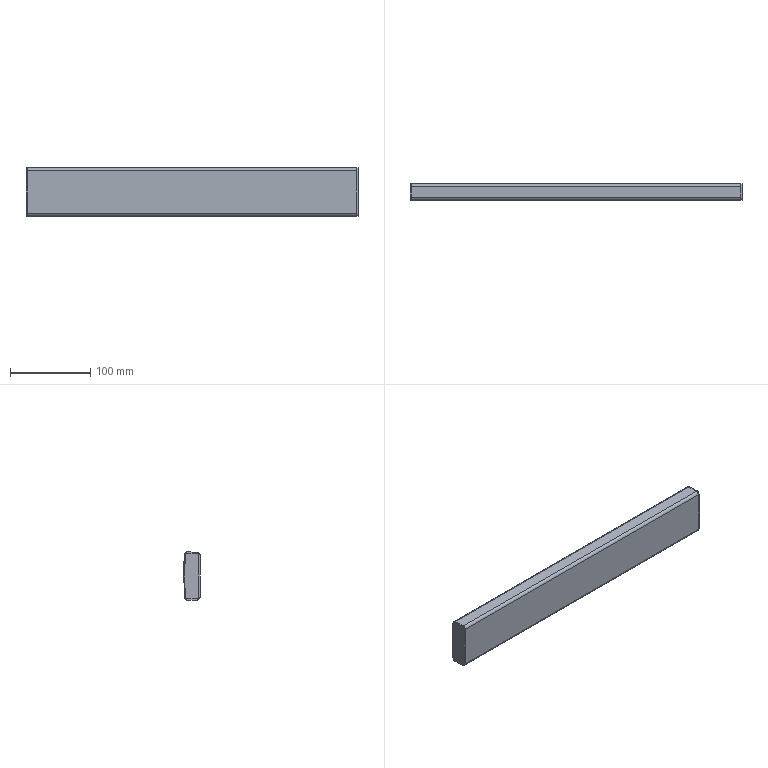Part | SolidWorks | features FlatPattern 3, EdgeFlange 2, SMBaseFlange 2, SheetMetal 2, HoleWzd 1, ICE 1, LPattern 1, MirrorSolid 1 | 5 solids | 74 faces | box 415 x 20 x 60 mm | volume 80765 mm3 | plane 54 | cylinder 20 | commonest cylinder face diameters 7 x12 4 x4 5 x4